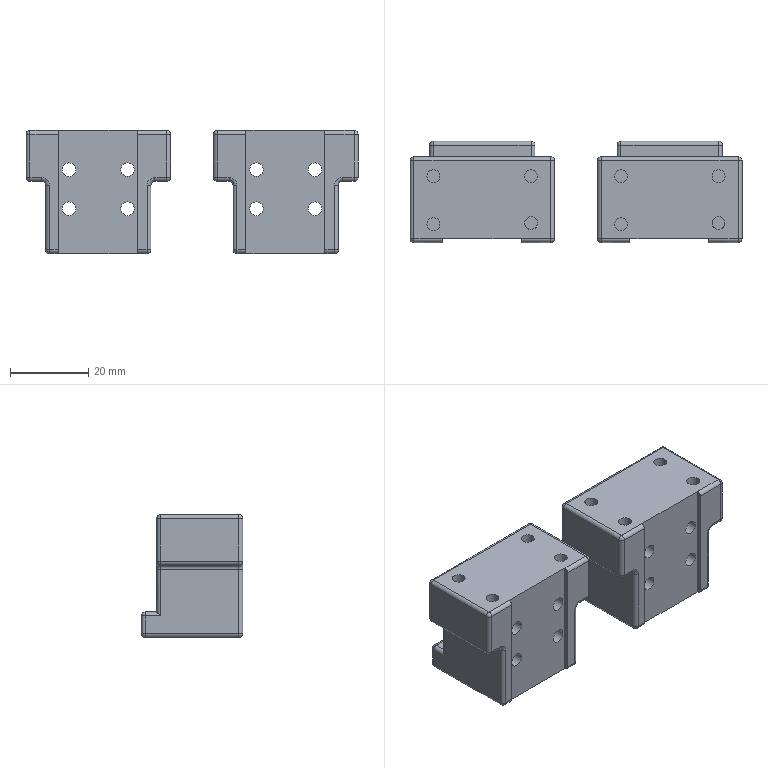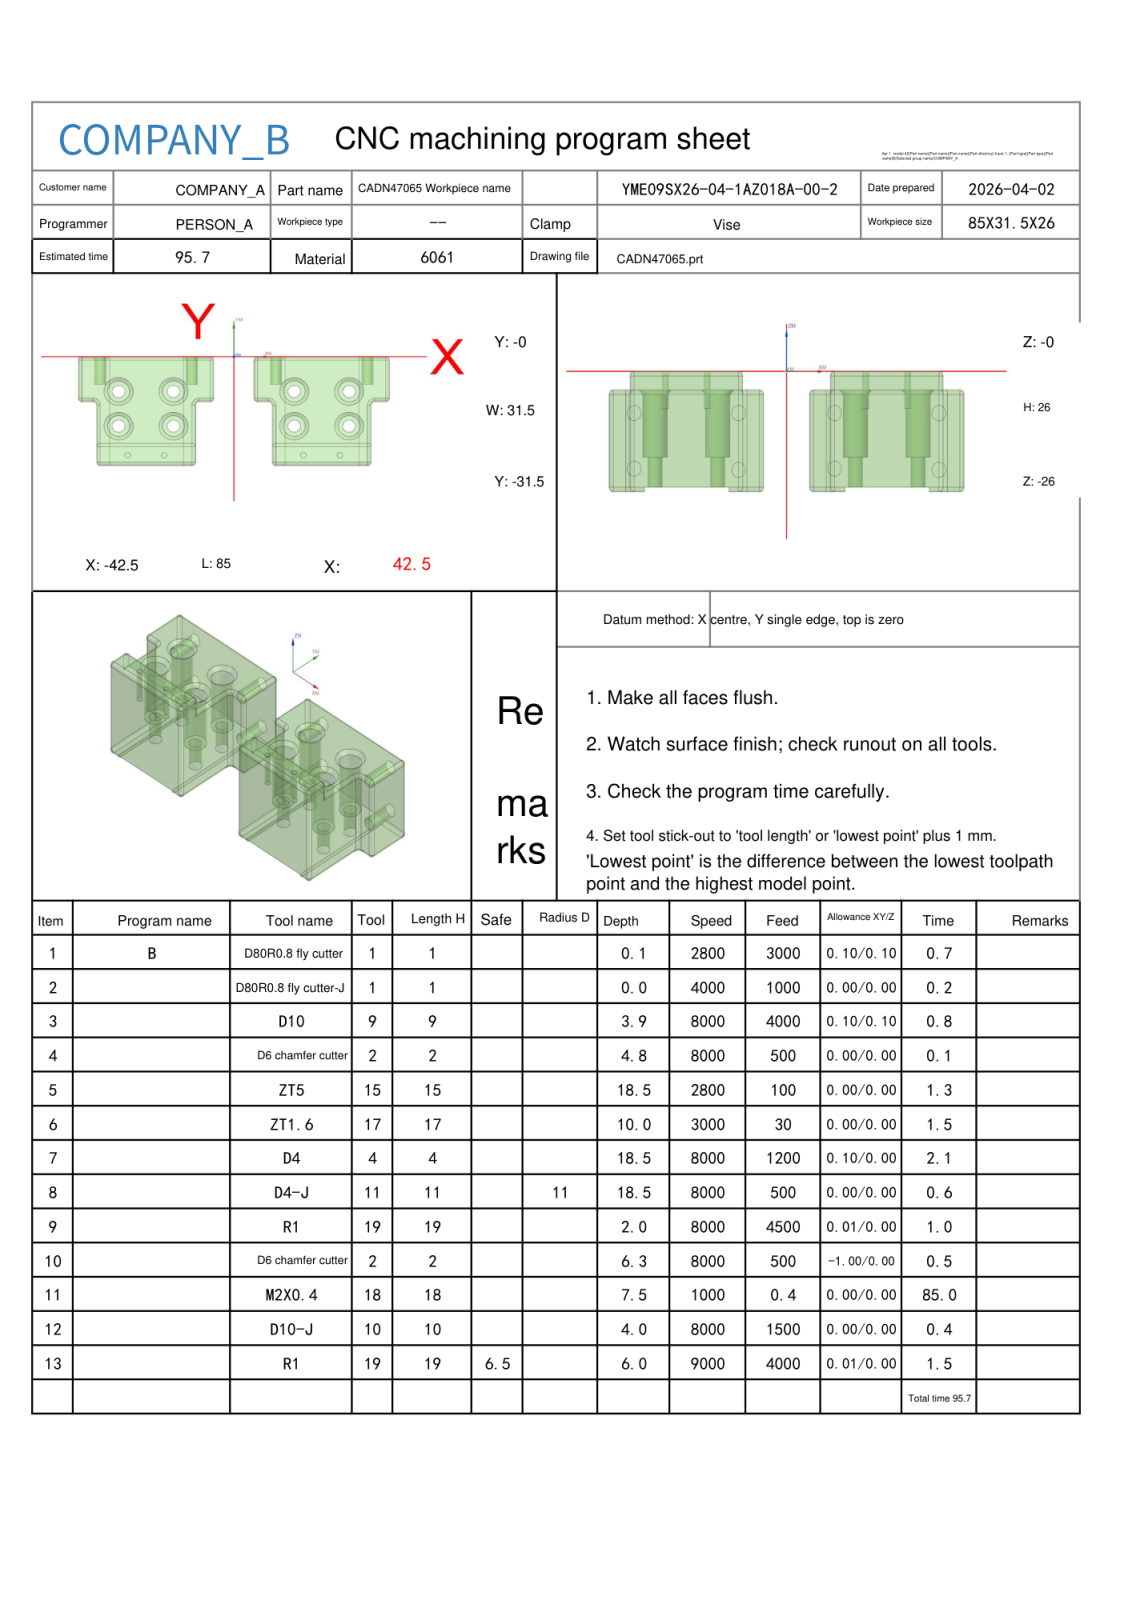NC program | NX | posted by the shop | part box 85 x 26 x 31.5 mm
Lines 1234 to 2575 of 12542:
N9 T19 M06
(R1  D=2. R=1. H=19 ce=0.01 di=0.00)
G00 G90 G54 X12.775 Y-25.799 M03 S8000
G43 H19 Z20.
M08
Z1.5
G01 X36.499 Z.257 F4500.
X36.539 Z.255
X36.614 Y-25.841 Z.25
X36.656 Y-25.916 Z.246
Y-25.955 Z.244
Y-30.5 Z.005
Y-30.54 Z.003
X36.613 Y-30.614 Z-.001
X36.538 Y-30.656 Z-.006
X36.498 Z-.008
X11.502
X11.5
G02 X11.344 Y-30.5 I0.0 J.156
G01 Y-25.955
G02 X11.5 Y-25.799 I.156 J0.0
G01 X36.499
G02 X36.656 Y-25.955 I0.0 J-.156
G01 Y-30.5
G02 X36.5 Y-30.656 I-.156 J0.0
G01 X36.498
X36.377 Y-30.686
X36.257
X36.137 Y-30.687
X36.017
X35.776 Y-30.688
X35.537
X35.056 Y-30.689
X34.575
X33.614 Y-30.692
X32.652 Y-30.694 Z-.009
X31.691 Y-30.696
X30.73 Y-30.698
X29.768 Y-30.7
X28.807 Y-30.702
X27.846 Y-30.704 Z-.01
X26.884 Y-30.707
X25.923 Y-30.708
X24.961 Y-30.711
X24. Y-30.712
X23.039 Y-30.714 Z-.011
X22.077 Y-30.716
X21.116 Y-30.718
X20.154 Y-30.72
X19.193 Y-30.721
X18.232 Y-30.724 Z-.012
X17.27 Y-30.725
X16.309 Y-30.727
X15.348 Y-30.728
X14.386 Y-30.731
X13.425 Y-30.732
X12.463 Y-30.734 Z-.013
X11.502 Y-30.735
X11.479
X11.456 Y-30.731
X11.434 Y-30.727
X11.412 Y-30.718
X11.391 Y-30.709
X11.371 Y-30.697
X11.351 Y-30.684
X11.335 Y-30.667
X11.318 Y-30.651
X11.305 Y-30.632
X11.292 Y-30.612
X11.283 Y-30.591
X11.274 Y-30.569
X11.269 Y-30.546
X11.264 Y-30.523
X11.263 Y-30.5
X11.265 Y-30.456
X11.267 Y-30.412
X11.264 Y-29.699
Y-28.985
X11.262 Y-28.228
Y-27.47 Z-.014
X11.26 Y-26.757
X11.259 Y-26.043
X11.258 Y-26.005
X11.259 Y-25.966
X11.255 Y-25.947
X11.258 Y-25.928
X11.263 Y-25.894
X11.275 Y-25.862
X11.284 Y-25.84
X11.297 Y-25.82
X11.311 Y-25.8
X11.328 Y-25.783
X11.345 Y-25.766
X11.365 Y-25.752
X11.385 Y-25.739
X11.407 Y-25.73
X11.429 Y-25.721
X11.453 Y-25.716
X11.476 Y-25.711
X11.5
X12.462 Y-25.709
X13.423 Y-25.708
X14.385 Y-25.706
X15.346 Y-25.704 Z-.015
X16.308 Y-25.703
X17.269 Y-25.701
X18.231 Y-25.699
X19.192 Y-25.697
X20.154 Y-25.696 Z-.016
X21.115 Y-25.694
X22.077 Y-25.693
X23.038 Y-25.691
X24. Y-25.69
X24.961 Y-25.689 Z-.017
X25.923 Y-25.687
X26.884 Y-25.686
X27.846 Y-25.684
X28.807 Y-25.691
X36.5 Z-.019
X36.525 Y-25.692
X36.551 Y-25.696
X36.576 Y-25.702
X36.601 Y-25.711
X36.624 Y-25.722
X36.647 Y-25.735
X36.668 Y-25.75
X36.687 Y-25.768
X36.704 Y-25.787
X36.72 Y-25.808
X36.733 Y-25.83
X36.744 Y-25.854
X36.753 Y-25.878
X36.76 Y-25.904
X36.763 Y-25.929
X36.765 Y-25.955
X36.761 Y-25.974
X36.749 Y-26.043
Y-30.412 Z-.02
X36.758 Y-30.488
X36.763 Y-30.529
X36.756 Y-30.566
X36.744 Y-30.602
X36.733 Y-30.626
X36.719 Y-30.648
X36.704 Y-30.669
X36.686 Y-30.688
X36.666 Y-30.706
X36.645 Y-30.721
X36.623 Y-30.735
X36.599 Y-30.745
X36.574 Y-30.754
X36.549 Y-30.76
X36.524 Y-30.764
X36.498 Y-30.765
X36.377 Y-30.792
X36.257
X36.137
X36.017
X35.777 Y-30.793
X35.537
X35.056 Y-30.794
X34.575 Y-30.796 Z-.021
X33.614 Y-30.797
X32.652 Y-30.799
X31.691 Y-30.801
X30.73 Y-30.803 Z-.022
X29.768 Y-30.804
X28.807 Y-30.807
X27.846 Y-30.808
X26.884 Y-30.81 Z-.023
X25.923 Y-30.812
X24.961 Y-30.814
X24. Y-30.815
X23.039 Y-30.817 Z-.024
X22.077 Y-30.819
X21.116 Y-30.821
X20.154 Y-30.822 Z-.025
X19.193 Y-30.824
X18.232 Y-30.826
X17.27 Y-30.827
X16.309 Y-30.829 Z-.026
X15.348 Y-30.831
X14.386 Y-30.832
X13.425 Y-30.834
X12.463 Y-30.835 Z-.027
X11.502 Y-30.837
X11.449 Y-30.833
X11.398 Y-30.821
X11.348 Y-30.802
X11.303 Y-30.774
X11.262 Y-30.74
X11.227 Y-30.699
X11.199 Y-30.654
X11.179 Y-30.605
X11.166 Y-30.553
X11.162 Y-30.5
X11.168 Y-30.456
Y-30.412
X11.166 Y-29.684
X11.165 Y-28.956 Z-.028
X11.164 Y-28.228
X11.162 Y-27.5
X11.161 Y-26.769
X11.159 Y-26.038
Y-25.988
X11.155 Y-25.939
X11.157 Y-25.917
X11.161 Y-25.886
X11.169 Y-25.855
X11.179 Y-25.825
X11.193 Y-25.797
X11.208 Y-25.769
X11.227 Y-25.743
X11.247 Y-25.719
X11.269 Y-25.697
X11.294 Y-25.677
X11.32 Y-25.66
X11.348 Y-25.644
X11.377 Y-25.632 Z-.029
X11.407 Y-25.622
X11.437 Y-25.615
X11.469 Y-25.61
X11.5 Y-25.609
X12.462 Y-25.608
X13.423 Y-25.606
X14.385 Y-25.605
X15.346 Y-25.603 Z-.03
X16.308 Y-25.602
X17.269 Y-25.599
X18.231 Y-25.598
X19.192 Y-25.596 Z-.031
X20.154 Y-25.595
X21.115 Y-25.593
X22.077 Y-25.592
X23.038 Y-25.591 Z-.032
X24. Y-25.589
X24.961 Y-25.588
X25.923 Y-25.586 Z-.033
X26.884 Y-25.585
X27.846 Y-25.583
X28.807 Y-25.582
X29.769 Y-25.58 Z-.034
X30.73 Y-25.579
X31.692 Y-25.577
X32.653 Y-25.576
X33.615 Y-25.574 Z-.035
X34.576 Y-25.573
X35.538 Y-25.572
X36.5 Y-25.57 Z-.036
X36.56 Y-25.575
X36.619 Y-25.589
X36.674 Y-25.612
X36.726 Y-25.643
X36.772 Y-25.682
X36.812 Y-25.728
X36.844 Y-25.78
X36.867 Y-25.836
X36.881 Y-25.895
X36.886 Y-25.955
X36.885 Y-25.972
X36.886 Y-26.008
X36.885 Y-26.044
X36.886 Y-26.772
X36.888 Y-27.5
Y-28.228
X36.881 Y-28.956 Z-.037
Y-30.412
X36.884 Y-30.437
X36.892 Y-30.461
Y-30.486
Y-30.51
X36.891 Y-30.527
X36.89 Y-30.543
X36.885 Y-30.579
X36.876 Y-30.614
X36.864 Y-30.648
X36.849 Y-30.681
X36.831 Y-30.712
X36.81 Y-30.741
X36.787 Y-30.769
X36.761 Y-30.794
X36.733 Y-30.817
X36.703 Y-30.837
X36.671 Y-30.854
X36.638 Y-30.868
X36.604 Y-30.879
X36.569 Y-30.887
X36.534 Y-30.892
X36.498 Y-30.894
X35.537 Y-30.895
X34.575 Y-30.897 Z-.038
X33.614 Y-30.898
X32.652 Y-30.9
X31.691 Y-30.902 Z-.039
X30.73 Y-30.903
X29.768 Y-30.905 Z-.04
X28.807 Y-30.907
X27.845 Y-30.908
X26.884 Y-30.91 Z-.041
X25.923 Y-30.912
X24.961 Y-30.913
X24. Y-30.915 Z-.042
X23.039 Y-30.916
X22.077 Y-30.918
X21.116 Y-30.92 Z-.043
X20.154 Y-30.922
X19.193 Y-30.923
X18.232 Y-30.925 Z-.044
X17.27 Y-30.926
X16.309 Y-30.928
X15.348 Y-30.93 Z-.045
X14.386 Y-30.931
X13.425 Y-30.933
X12.463 Y-30.935 Z-.046
X11.502 Y-30.936
X11.468 Y-30.935
X11.434 Y-30.931
X11.4 Y-30.925
X11.367 Y-30.915
X11.334 Y-30.904
X11.303 Y-30.89
X11.273 Y-30.873
X11.245 Y-30.854
X11.217 Y-30.833
X11.192 Y-30.81
X11.168 Y-30.785
X11.147 Y-30.757
X11.128 Y-30.729
X11.111 Y-30.699
X11.096 Y-30.668
X11.085 Y-30.635
X11.075 Y-30.602
X11.068 Y-30.569
X11.064 Y-30.534
X11.063 Y-30.5
X11.064 Y-30.456
Y-30.412
X11.063 Y-29.684 Z-.047
X11.062 Y-28.956
X11.061 Y-28.228
X11.06 Y-27.5
X11.059 Y-26.771 Z-.048
X11.058 Y-26.043
X11.057 Y-25.993
X11.055 Y-25.944
X11.058 Y-25.909
X11.062 Y-25.875
X11.07 Y-25.842
X11.08 Y-25.809
X11.092 Y-25.777
X11.107 Y-25.746
X11.125 Y-25.716
X11.144 Y-25.688
X11.166 Y-25.661
X11.189 Y-25.636
X11.215 Y-25.613
X11.242 Y-25.592
X11.271 Y-25.573
X11.301 Y-25.557
X11.332 Y-25.542
X11.365 Y-25.531
X11.398 Y-25.521
X11.432 Y-25.515
X11.466 Y-25.511
X11.5 Y-25.509
X12.462 Y-25.508
X13.423 Y-25.507 Z-.049
X14.385 Y-25.505
X15.346 Y-25.504
X16.308 Y-25.502 Z-.05
X17.269 Y-25.501
X18.231 Y-25.499
X19.192 Y-25.498 Z-.051
X20.154 Y-25.496
X21.115 Y-25.495 Z-.052
X22.077 Y-25.493
X23.038 Y-25.492
X24. Y-25.49 Z-.053
X24.961 Y-25.489
X25.923 Y-25.488
X26.884 Y-25.486 Z-.054
X27.846 Y-25.485
X28.807 Y-25.483
X29.769 Y-25.482 Z-.055
X30.73 Y-25.48
X31.692 Y-25.479
X32.653 Y-25.478 Z-.056
X33.615 Y-25.476
X34.576 Y-25.475
X35.538 Y-25.473 Z-.057
X36.5 Y-25.472
X36.537 Y-25.473
X36.575 Y-25.477
X36.613 Y-25.485
X36.649 Y-25.495
X36.685 Y-25.508
X36.719 Y-25.524
X36.753 Y-25.542
X36.784 Y-25.563
X36.814 Y-25.587
X36.842 Y-25.613
X36.868 Y-25.64
X36.892 Y-25.67
X36.913 Y-25.702
X36.932 Y-25.735
X36.948 Y-25.77
X36.961 Y-25.805
X36.971 Y-25.842
X36.979 Y-25.879
X36.983 Y-25.917
X36.985 Y-25.955
X36.98 Y-25.999
Y-26.043
X36.982 Y-26.771 Z-.058
X36.983 Y-27.5
X36.984 Y-28.228
X36.985 Y-28.956
X36.986 Y-29.684 Z-.059
X36.987 Y-30.412
Y-30.462
X36.991 Y-30.513
X36.989 Y-30.551
X36.984 Y-30.589
X36.975 Y-30.626
X36.964 Y-30.662
X36.95 Y-30.698
X36.934 Y-30.732
X36.914 Y-30.765
X36.893 Y-30.796
X36.869 Y-30.826
X36.842 Y-30.853
X36.814 Y-30.879
X36.784 Y-30.902
X36.752 Y-30.923
X36.718 Y-30.941
X36.684 Y-30.957
X36.648 Y-30.97
X36.611 Y-30.98
X36.574 Y-30.987
X36.536 Y-30.991
X36.498 Y-30.993
X35.537 Y-30.994 Z-.06
X34.575 Y-30.996
X33.614 Y-30.997
X32.652 Y-30.999 Z-.061
X31.691 Y-31.001
X30.73 Y-31.002 Z-.062
X29.768 Y-31.004
X28.807 Y-31.005
X27.845 Y-31.007 Z-.063
X26.884 Y-31.008
X25.923 Y-31.011 Z-.064
X24.961 Y-31.012
X24. Y-31.014 Z-.065
X23.039 Y-31.015
X22.077 Y-31.017
X21.116 Y-31.018 Z-.066
X20.154 Y-31.02
X19.193 Y-31.021 Z-.067
X18.232 Y-31.023
X17.27 Y-31.024
X16.309 Y-31.026 Z-.068
X15.348 Y-31.027
X14.386 Y-31.029 Z-.069
X13.425 Y-31.031
X12.463 Y-31.032
X11.502 Y-31.034 Z-.07
X11.467 Y-31.033
X11.432 Y-31.03
X11.398 Y-31.024
X11.364 Y-31.016
X11.33 Y-31.006
X11.297 Y-30.994
X11.265 Y-30.98
X11.234 Y-30.963
X11.204 Y-30.945
X11.176 Y-30.925
X11.148 Y-30.903
X11.123 Y-30.879
X11.099 Y-30.853
X11.076 Y-30.826
X11.056 Y-30.798
X11.037 Y-30.768
X11.021 Y-30.737
X11.006 Y-30.705
X10.993 Y-30.672
X10.983 Y-30.639
X10.975 Y-30.605
X10.97 Y-30.57
X10.966 Y-30.535
X10.965 Y-30.5
X10.967 Y-29.743 Z-.071
X10.965 Y-28.985
X10.964 Y-28.228
X10.963 Y-27.47 Z-.072
X10.962 Y-26.713
X10.958 Y-25.955
X10.959 Y-25.92
X10.962 Y-25.884
X10.968 Y-25.849
X10.976 Y-25.815
X10.986 Y-25.781
X10.999 Y-25.747
X11.013 Y-25.715
X11.03 Y-25.684
X11.049 Y-25.654
X11.069 Y-25.625
X11.092 Y-25.597
X11.116 Y-25.571
X11.142 Y-25.547
X11.169 Y-25.524
X11.198 Y-25.503
X11.229 Y-25.485
X11.26 Y-25.468
X11.292 Y-25.453
X11.326 Y-25.441
X11.36 Y-25.43 Z-.073
X11.394 Y-25.422
X11.429 Y-25.416
X11.465 Y-25.413
X11.5 Y-25.412
X12.462 Y-25.411
X13.423 Y-25.409
X14.385 Y-25.408 Z-.074
X15.346 Y-25.406
X16.308 Y-25.405 Z-.075
X17.269 Y-25.403
X18.231 Y-25.402
X19.192 Y-25.4 Z-.076
X20.154 Y-25.399
X21.115 Y-25.397 Z-.077
X22.077 Y-25.396
X23.038 Y-25.394 Z-.078
X24. Y-25.393
X24.961 Y-25.391
X25.923 Y-25.39 Z-.079
X26.884 Y-25.389
X27.846 Y-25.387 Z-.08
X28.807 Y-25.386
X29.769 Y-25.384
X30.73 Y-25.383 Z-.081
X31.692 Y-25.381
X32.653 Y-25.38 Z-.082
X33.615 Y-25.378
X34.576 Y-25.377 Z-.083
X35.538 Y-25.375
X36.5 Y-25.374
X36.538 Y-25.375
X36.575 Y-25.379
X36.613 Y-25.385
X36.65 Y-25.394
X36.687 Y-25.404
X36.722 Y-25.418
X36.757 Y-25.433
X36.79 Y-25.452
X36.823 Y-25.471
X36.854 Y-25.494 Z-.084
X36.883 Y-25.518
X36.911 Y-25.544
X36.937 Y-25.571
X36.961 Y-25.601
X36.984 Y-25.632
X37.004 Y-25.664
X37.022 Y-25.698
X37.038 Y-25.732
X37.051 Y-25.768
X37.062 Y-25.805
X37.071 Y-25.842
X37.077 Y-25.879
X37.081 Y-25.917
X37.083 Y-25.955
X37.084 Y-26.713
Y-27.47
X37.086 Y-28.228 Z-.085
X37.087 Y-28.985
X37.088 Y-29.743
X37.089 Y-30.5 Z-.086
X37.088 Y-30.539
X37.084 Y-30.577
X37.078 Y-30.615
X37.069 Y-30.653
X37.058 Y-30.69
X37.044 Y-30.726
X37.028 Y-30.761
X37.01 Y-30.795
X36.99 Y-30.828
X36.967 Y-30.86
X36.943 Y-30.89
X36.916 Y-30.918
X36.888 Y-30.944
X36.858 Y-30.969
X36.826 Y-30.991
X36.794 Y-31.012
X36.759 Y-31.03
X36.724 Y-31.046
X36.688 Y-31.059
X36.651 Y-31.071
X36.613 Y-31.079
X36.575 Y-31.086
X36.537 Y-31.089
X36.498 Y-31.09
X35.537 Y-31.092 Z-.087
X34.575 Y-31.094
X33.614 Y-31.095 Z-.088
X32.652 Y-31.097
X31.691 Y-31.098 Z-.089
X30.73 Y-31.1
X29.768 Y-31.101
X28.807 Y-31.103 Z-.09
X27.845 Y-31.104
X26.884 Y-31.106 Z-.091
X25.923 Y-31.107
X24.961 Y-31.109 Z-.092
X24. Y-31.11
X23.039 Y-31.112 Z-.093
X22.077 Y-31.113
X21.116 Y-31.115 Z-.094
X20.154 Y-31.116
X19.193 Y-31.118 Z-.095
X18.232 Y-31.119
X17.27 Y-31.121 Z-.096
X16.309 Y-31.122
X15.348 Y-31.124 Z-.097
X14.386 Y-31.125
X13.425 Y-31.127 Z-.098
X12.463 Y-31.128
X11.502 Y-31.13 Z-.099
X11.431 Y-31.127
X11.362 Y-31.115
X11.293 Y-31.096
X11.228 Y-31.069
X11.166 Y-31.035
X11.108 Y-30.994
X11.055 Y-30.947
X11.007 Y-30.894
X10.966 Y-30.836
X10.932 Y-30.774
X10.904 Y-30.709
X10.884 Y-30.641
X10.872 Y-30.57
X10.868 Y-30.498
X10.869 Y-30.455
X10.87 Y-30.412
X10.868 Y-29.699 Z-.1
Y-28.985
X10.867 Y-28.228
X10.865 Y-27.47 Z-.101
X10.864 Y-26.757
X10.863 Y-26.043
Y-26.
X10.861 Y-25.957
X10.862 Y-25.929
X10.867 Y-25.87
X10.877 Y-25.813 Z-.102
X10.897 Y-25.744
X10.924 Y-25.678
X10.959 Y-25.615
X11. Y-25.556
X11.048 Y-25.503
X11.101 Y-25.455
X11.16 Y-25.414
X11.223 Y-25.379
X11.289 Y-25.351
X11.358 Y-25.331
X11.428 Y-25.319
X11.5 Y-25.315
X12.462 Y-25.314
X13.423 Y-25.312 Z-.103
X14.385 Y-25.311
X15.346 Y-25.309 Z-.104
X16.308 Y-25.308
X17.269 Y-25.307 Z-.105
X18.231 Y-25.305
X19.192 Y-25.304 Z-.106
X20.154 Y-25.302
X21.115 Y-25.301 Z-.107
X22.077 Y-25.299
X23.038 Y-25.298 Z-.108
X24. Y-25.296
X24.961 Y-25.295 Z-.109
X25.923 Y-25.294
X26.884 Y-25.293 Z-.11
X27.846 Y-25.291
X28.807 Y-25.29 Z-.111
X29.769 Y-25.288
X30.73 Y-25.287 Z-.112
X31.692 Y-25.285
X32.653 Y-25.284 Z-.113
X33.615 Y-25.282
X34.577 Y-25.281 Z-.114
X35.538 Y-25.28
X36.5 Y-25.279 Z-.115
X36.575 Y-25.283
X36.65 Y-25.295
X36.723 Y-25.316
X36.793 Y-25.345
X36.86 Y-25.382
X36.922 Y-25.425
X36.979 Y-25.476
X37.03 Y-25.533
X37.074 Y-25.595
X37.111 Y-25.661
X37.14 Y-25.731
X37.161 Y-25.804
X37.174 Y-25.879
X37.178 Y-25.955
X37.175 Y-25.999
Y-26.043
X37.176 Y-26.757
X37.177 Y-27.47 Z-.116
X37.178 Y-28.228
X37.179 Y-28.985 Z-.117
X37.18 Y-29.699
X37.181 Y-30.412
Y-30.454
X37.185 Y-30.497
X37.184 Y-30.513
Y-30.529
X37.179 Y-30.591
X37.168 Y-30.653
X37.147 Y-30.727
X37.117 Y-30.798
X37.08 Y-30.865 Z-.118
X37.035 Y-30.928
X36.984 Y-30.986
X36.927 Y-31.037
X36.864 Y-31.081
X36.796 Y-31.119
X36.725 Y-31.148
X36.651 Y-31.169
X36.575 Y-31.182
X36.498 Y-31.186
X35.537 Y-31.188
X34.575 Y-31.189 Z-.119
X33.614 Y-31.191 Z-.12
X32.652 Y-31.192
X31.691 Y-31.194 Z-.121
X30.73 Y-31.195
X29.768 Y-31.197 Z-.122
X28.807 Y-31.198
X27.845 Y-31.2 Z-.123
X26.884 Y-31.201
X25.923 Y-31.203 Z-.124
X24.961 Y-31.204
X24. Y-31.206 Z-.125
X23.039 Y-31.207 Z-.126
X22.077 Y-31.209
X21.116 Y-31.21 Z-.127
X20.154 Y-31.212
X19.193 Y-31.213 Z-.128
X18.232 Y-31.215
X17.27 Y-31.216 Z-.129
X16.309 Y-31.218
X15.348 Y-31.219 Z-.13
X14.386 Y-31.22 Z-.131
X13.425 Y-31.222
X12.463 Y-31.223 Z-.132
X11.502 Y-31.225
X11.421 Y-31.221
X11.34 Y-31.207
X11.262 Y-31.185
X11.187 Y-31.154
X11.115 Y-31.115
X11.049 Y-31.068
X10.988 Y-31.014
X10.933 Y-30.953 Z-.133
X10.886 Y-30.887
X10.846 Y-30.815
X10.815 Y-30.74
X10.792 Y-30.662
X10.778 Y-30.581
X10.774 Y-30.5
X10.775 Y-30.456
Y-30.412
X10.774 Y-29.684
X10.773 Y-28.956 Z-.134
X10.772 Y-28.228
X10.771 Y-27.5 Z-.135
X10.769 Y-26.771
X10.768 Y-26.043
Y-25.998
X10.767 Y-25.954
Y-25.925
X10.775 Y-25.845
X10.791 Y-25.766 Z-.136
X10.816 Y-25.69
X10.849 Y-25.617
X10.889 Y-25.548
X10.937 Y-25.484
X10.992 Y-25.426
X11.052 Y-25.373
X11.118 Y-25.328
X11.189 Y-25.29
X11.263 Y-25.26
X11.34 Y-25.238
X11.42 Y-25.225
X11.5 Y-25.22
X12.461 Y-25.219 Z-.137
X13.423 Y-25.218
X14.384 Y-25.216 Z-.138
X15.346 Y-25.215
X16.307 Y-25.213 Z-.139
X17.269 Y-25.212
X18.23 Y-25.211 Z-.14
X19.192 Y-25.209
X20.153 Y-25.208 Z-.141
X21.115 Y-25.207 Z-.142
X22.077 Y-25.205
X23.038 Y-25.204 Z-.143
X24. Y-25.202
X24.961 Y-25.201 Z-.144
X25.923 Y-25.199
X26.884 Y-25.198 Z-.145
X27.846 Y-25.197
X28.807 Y-25.196 Z-.146
X29.769 Y-25.194
X30.73 Y-25.193 Z-.147
X31.692 Y-25.191 Z-.148
X32.653 Y-25.19
X33.615 Y-25.189 Z-.149
X34.576 Y-25.188
X35.538 Y-25.186 Z-.15
X36.5 Y-25.185
X36.586 Y-25.189
X36.671 Y-25.204
X36.754 Y-25.227
X36.834 Y-25.261 Z-.151
X36.91 Y-25.302
X36.981 Y-25.352
X37.045 Y-25.41
X37.103 Y-25.474
X37.153 Y-25.545
X37.195 Y-25.62
X37.229 Y-25.7
X37.253 Y-25.783
X37.267 Y-25.869
X37.272 Y-25.955
Y-25.999
Y-26.043
X37.274 Y-26.771
Y-27.5 Z-.152
X37.276 Y-28.228
Y-28.956 Z-.153
X37.278 Y-29.684
X37.279 Y-30.412 Z-.154
Y-30.456
Y-30.5
X37.278 Y-30.516
Y-30.533
X37.27 Y-30.617
X37.253 Y-30.701
X37.226 Y-30.782
X37.191 Y-30.86
X37.148 Y-30.933
X37.097 Y-31.001
X37.039 Y-31.063
X36.974 Y-31.119
X36.904 Y-31.167
X36.828 Y-31.207
X36.749 Y-31.239
X36.667 Y-31.262
X36.583 Y-31.276
X36.498 Y-31.28
X35.537 Y-31.282 Z-.155
X34.575 Y-31.283 Z-.156
X33.614 Y-31.285
X32.652 Y-31.286 Z-.157
X31.691 Y-31.288
X30.73 Y-31.289 Z-.158
X29.768 Y-31.29 Z-.159
X28.807 Y-31.292
X27.845 Y-31.293 Z-.16
X26.884 Y-31.295
X25.923 Y-31.296 Z-.161
X24.961 Y-31.297 Z-.162
X24. Y-31.299
X23.039 Y-31.3 Z-.163
X22.077 Y-31.302 Z-.164
X21.116 Y-31.303
X20.154 Y-31.305 Z-.165
X19.193 Y-31.306
X18.232 Y-31.308 Z-.166
X17.27 Y-31.309 Z-.167
X16.309 Y-31.31
X15.347 Y-31.312 Z-.168
X14.386 Y-31.313
X13.425 Y-31.314 Z-.169
X12.463 Y-31.316 Z-.17
X11.502 Y-31.317
X11.456 Y-31.316
X11.41 Y-31.312
X11.365 Y-31.306
X11.32 Y-31.297
X11.275 Y-31.286
X11.231 Y-31.272
X11.188 Y-31.256
X11.147 Y-31.237
X11.106 Y-31.217 Z-.171
X11.066 Y-31.193
X11.028 Y-31.168
X10.991 Y-31.14
X10.956 Y-31.111
X10.922 Y-31.079
X10.89 Y-31.046
X10.861 Y-31.011
X10.833 Y-30.974
X10.807 Y-30.936
X10.784 Y-30.897
X10.763 Y-30.856
X10.744 Y-30.814
X10.727 Y-30.771
X10.713 Y-30.727
X10.702 Y-30.682
X10.693 Y-30.637
X10.686 Y-30.592
X10.682 Y-30.546
X10.681 Y-30.5
Y-29.743 Z-.172
X10.68 Y-28.985
X10.679 Y-28.228 Z-.173
X10.678 Y-27.47
X10.677 Y-26.713
X10.674 Y-25.955 Z-.174
X10.675 Y-25.909
X10.679 Y-25.863
X10.686 Y-25.817
X10.695 Y-25.771
X10.706 Y-25.727
X10.72 Y-25.682
X10.737 Y-25.639
X10.756 Y-25.597
X10.777 Y-25.555
X10.8 Y-25.515
X10.826 Y-25.477
X10.854 Y-25.44
X10.884 Y-25.404
X10.916 Y-25.371
X10.949 Y-25.339
X10.985 Y-25.309
X11.022 Y-25.281
X11.06 Y-25.255
X11.1 Y-25.231 Z-.175
X11.141 Y-25.21
X11.184 Y-25.191
X11.227 Y-25.174
X11.271 Y-25.16
X11.316 Y-25.149
X11.362 Y-25.139
X11.408 Y-25.133
X11.454 Y-25.129
X11.5 Y-25.128
X12.462 Y-25.126
X13.423 Y-25.125 Z-.176
X14.385 Y-25.124 Z-.177
X15.346 Y-25.122
X16.308 Y-25.121 Z-.178
X17.269 Y-25.12
X18.231 Y-25.118 Z-.179
X19.192 Y-25.117 Z-.18
X20.154 Y-25.116
X21.115 Y-25.114 Z-.181
X22.077 Y-25.113 Z-.182
X23.038 Y-25.112
X24. Y-25.11 Z-.183
X24.961 Y-25.109
X25.923 Y-25.107 Z-.184
X26.884 Y-25.106 Z-.185
X27.846 Y-25.105
X28.807 Y-25.104 Z-.186
X29.769 Y-25.102
X30.73 Y-25.101 Z-.187
X31.692 Y-25.099 Z-.188
X32.653
X33.615 Y-25.097 Z-.189
X34.577 Y-25.096
X35.538 Y-25.094 Z-.19
X36.5 Y-25.093 Z-.191
X36.548 Y-25.094
X36.596 Y-25.098
X36.644 Y-25.105
X36.691 Y-25.114
X36.738 Y-25.126
X36.784 Y-25.141
X36.83 Y-25.158
X36.874 Y-25.178
X36.917 Y-25.2
X36.959 Y-25.225
X36.999 Y-25.251
X37.038 Y-25.281
X37.075 Y-25.312
X37.11 Y-25.345
X37.144 Y-25.38
X37.175 Y-25.417
X37.204 Y-25.456
X37.231 Y-25.496
X37.256 Y-25.537
X37.278 Y-25.581
X37.298 Y-25.625
X37.315 Y-25.67
X37.33 Y-25.716
X37.342 Y-25.763
X37.352 Y-25.811
X37.358 Y-25.859 Z-.192
X37.363 Y-25.907
X37.364 Y-25.955
X37.363 Y-26.713
X37.364 Y-27.47 Z-.193
X37.365 Y-28.228
X37.366 Y-28.985 Z-.194
X37.367 Y-29.743
X37.37 Y-30.5
X37.369 Y-30.549 Z-.195
X37.365 Y-30.598
X37.358 Y-30.646
X37.349 Y-30.694
X37.336 Y-30.741
X37.322 Y-30.788
X37.304 Y-30.834
X37.284 Y-30.878
X37.262 Y-30.922
X37.237 Y-30.964
X37.21 Y-31.005
X37.18 Y-31.044
X37.149 Y-31.081
X37.115 Y-31.117
X37.08 Y-31.15
X37.042 Y-31.182
X37.003 Y-31.211
X36.962 Y-31.239
X36.92 Y-31.263
X36.877 Y-31.286
X36.832 Y-31.306
X36.786 Y-31.323
X36.74 Y-31.338
X36.692 Y-31.35
X36.644 Y-31.36
X36.596 Y-31.367
X36.547 Y-31.371
X36.498 Y-31.372
X35.537 Y-31.373 Z-.196
X34.575 Y-31.375 Z-.197
X33.614 Y-31.376
X32.652 Y-31.378 Z-.198
X31.691 Y-31.379 Z-.199
X30.73 Y-31.38
X29.768 Y-31.382 Z-.2
X28.807 Y-31.383 Z-.201
X27.845 Y-31.385
X26.884 Y-31.386 Z-.202
X25.923 Y-31.387 Z-.203
X24.961 Y-31.388
X24. Y-31.39 Z-.204
X23.039 Y-31.391 Z-.205
X22.077 Y-31.393
X21.116 Y-31.394 Z-.206
X20.154 Y-31.396 Z-.207
X19.193 Y-31.397
X18.232 Y-31.398 Z-.208
X17.27 Y-31.399 Z-.209
X16.309 Y-31.401
X15.347 Y-31.402 Z-.21
X14.386 Y-31.404 Z-.211
X13.425 Y-31.405 Z-.212
X12.463 Y-31.406
X11.502 Y-31.408 Z-.213
X11.413 Y-31.404
X11.325 Y-31.391
X11.238 Y-31.369
X11.154 Y-31.34
X11.073 Y-31.302
X10.996 Y-31.256
X10.924 Y-31.203
X10.858 Y-31.143
X10.798 Y-31.077
X10.745 Y-31.006
X10.699 Y-30.929 Z-.214
X10.66 Y-30.848
X10.63 Y-30.764
X10.608 Y-30.678
X10.595 Y-30.589
X10.59 Y-30.5
X10.591 Y-30.456
Y-30.412
X10.59 Y-29.699
X10.589 Y-28.985 Z-.215
X10.588 Y-28.228
X10.587 Y-27.47 Z-.216
X10.586 Y-26.757
X10.585 Y-26.043 Z-.217
Y-26.
X10.584 Y-25.937
X10.589 Y-25.856
X10.601 Y-25.777
X10.623 Y-25.689
X10.653 Y-25.604
X10.692 Y-25.523
X10.738 Y-25.446
X10.791 Y-25.374
X10.852 Y-25.307 Z-.218
X10.918 Y-25.246
X10.991 Y-25.192
X11.068 Y-25.146
X11.149 Y-25.107
X11.234 Y-25.077
X11.321 Y-25.055
X11.41 Y-25.042
X11.5 Y-25.037
X12.462 Y-25.036 Z-.219
X13.423 Y-25.035
X14.385 Y-25.033 Z-.22
X15.346 Y-25.032 Z-.221
X16.308 Y-25.031
X17.269 Y-25.03 Z-.222
X18.231 Y-25.028 Z-.223
X19.192 Y-25.027
X20.154 Y-25.026 Z-.224
X21.115 Y-25.024 Z-.225
X22.077 Y-25.023
X23.038 Y-25.022 Z-.226
X24. Y-25.02 Z-.227
X24.961 Y-25.019
X25.923 Y-25.018 Z-.228
X26.884 Y-25.017 Z-.229
X27.846 Y-25.015 Z-.23
X28.807 Y-25.014
X29.769 Y-25.013 Z-.231
X30.73 Y-25.012 Z-.232
X31.692 Y-25.01
X32.654 Y-25.009 Z-.233
X33.615 Y-25.008 Z-.234
X34.577 Y-25.006
X35.538 Y-25.005 Z-.235
X36.5 Y-25.004 Z-.236
X36.593 Y-25.008
X36.685 Y-25.022
X36.776 Y-25.044
X36.864 Y-25.076
X36.949 Y-25.115
X37.029 Y-25.163
X37.104 Y-25.219
X37.173 Y-25.282
X37.236 Y-25.351
X37.292 Y-25.426
X37.34 Y-25.506
X37.38 Y-25.591
X37.412 Y-25.679
X37.435 Y-25.769
X37.449 Y-25.862 Z-.237
X37.454 Y-25.955
Y-25.999
X37.453 Y-26.043
X37.455 Y-26.757
Y-27.47 Z-.238
X37.457 Y-28.228
Y-28.985 Z-.239
X37.458 Y-29.699
X37.459 Y-30.412 Z-.24
Y-30.454
Y-30.52
X37.454 Y-30.604
X37.441 Y-30.687
X37.418 Y-30.779
X37.387 Y-30.868
X37.346 Y-30.953
X37.298 Y-31.034
X37.242 Y-31.11
X37.178 Y-31.18
X37.108 Y-31.243
X37.033 Y-31.3
X36.952 Y-31.348 Z-.241
X36.866 Y-31.388
X36.777 Y-31.42
X36.686 Y-31.443
X36.592 Y-31.457
X36.498 Y-31.462
X35.537 Y-31.463 Z-.242
X34.575 Y-31.464
X33.614 Y-31.466 Z-.243
X32.652 Y-31.467 Z-.244
X31.691 Y-31.468 Z-.245
X30.73 Y-31.469
X29.768 Y-31.471 Z-.246
X28.807 Y-31.472 Z-.247
X27.845 Y-31.474
X26.884 Y-31.475 Z-.248
X25.923 Y-31.476 Z-.249
X24.961 Y-31.477 Z-.25
X24. Y-31.479
X23.039 Y-31.48 Z-.251
X22.077 Y-31.482 Z-.252
X21.116 Z-.253
X20.154 Y-31.484
X19.193 Y-31.485 Z-.254
X18.232 Y-31.487 Z-.255
X17.27 Y-31.488
X16.309 Y-31.489 Z-.256
X15.347 Y-31.49 Z-.257
X14.386 Y-31.492 Z-.258
X13.425 Y-31.493
X12.463 Y-31.495 Z-.259
X11.502 Y-31.496 Z-.26
X11.453 Y-31.495
X11.404 Y-31.491
X11.356 Y-31.486
X11.307 Y-31.477
X11.26 Y-31.467
X11.212 Y-31.454
X11.166 Y-31.439
X11.12 Y-31.421
X11.075 Y-31.401
X11.032 Y-31.379
X10.989 Y-31.355
X10.947 Y-31.329
X10.907 Y-31.301
X10.869 Y-31.271
X10.831 Y-31.239
X10.796 Y-31.205
X10.762 Y-31.17 Z-.261
X10.73 Y-31.133
X10.7 Y-31.095
X10.671 Y-31.055
X10.645 Y-31.013
X10.621 Y-30.971
X10.599 Y-30.927
X10.579 Y-30.882
X10.561 Y-30.836
X10.546 Y-30.79
X10.532 Y-30.743
X10.522 Y-30.695
X10.513 Y-30.647
X10.507 Y-30.598
X10.503 Y-30.549
X10.502 Y-30.5
X10.503 Y-30.456
Y-30.412
X10.502 Y-29.684 Z-.262
X10.501 Y-28.956
X10.5 Y-28.228 Z-.263
Y-27.5
X10.499 Y-26.771 Z-.264
X10.498 Y-26.043
Y-25.998 Z-.265
X10.496 Y-25.935
X10.503 Y-25.838
X10.519 Y-25.742
X10.544 Y-25.648
X10.578 Y-25.557
X10.621 Y-25.469
X10.672 Y-25.386
X10.73 Y-25.309
X10.796 Y-25.237
X10.869 Y-25.173
X10.948 Y-25.115
X11.032 Y-25.066
X11.12 Y-25.024
X11.212 Y-24.992 Z-.266
X11.306 Y-24.968
X11.402 Y-24.954
X11.5 Y-24.949
X12.461 Y-24.948
X13.423 Y-24.947 Z-.267
X14.384 Y-24.945 Z-.268
X15.346 Y-24.944 Z-.269
X16.307 Y-24.943
X17.269 Y-24.942 Z-.27
X18.23 Y-24.94 Z-.271
X19.192 Y-24.939 Z-.272
X20.153 Y-24.938
X21.115 Y-24.937 Z-.273
X22.077 Y-24.935 Z-.274
X23.038 Y-24.934 Z-.275
X24. Y-24.933
X24.961 Y-24.932 Z-.276
X25.923 Y-24.93 Z-.277
X26.884 Y-24.929
X27.846 Y-24.928 Z-.278
X28.807 Y-24.927 Z-.279
X29.769 Y-24.925 Z-.28
X30.73 Y-24.924
X31.692 Y-24.923 Z-.281
X32.653 Y-24.922 Z-.282
X33.615 Y-24.92 Z-.283
X34.576 Y-24.919
X35.538 Y-24.918 Z-.284
X36.5 Y-24.917 Z-.285
X36.551 Y-24.918
X36.601 Y-24.922
X36.652 Y-24.928
X36.702 Y-24.937
X36.752 Y-24.947
X36.801 Y-24.961
X36.85 Y-24.977
X36.897 Y-24.995
X36.944 Y-25.016
X36.989 Y-25.039
X37.034 Y-25.064
X37.077 Y-25.091
X37.119 Y-25.12
X37.159 Y-25.152
X37.198 Y-25.185
X37.235 Y-25.22
X37.27 Y-25.257
X37.303 Y-25.296
X37.335 Y-25.336 Z-.286
X37.364 Y-25.378
X37.392 Y-25.421
X37.417 Y-25.465
X37.44 Y-25.511
X37.461 Y-25.557
X37.479 Y-25.605
X37.495 Y-25.653
X37.509 Y-25.702
X37.52 Y-25.752
X37.529 Y-25.803
X37.535 Y-25.853
X37.539 Y-25.904
X37.541 Y-25.955
X37.538 Y-25.999
X37.541 Y-28.228 Z-.288
X37.542 Y-28.956
X37.543 Y-29.684 Z-.289
X37.544 Y-30.412
Y-30.456
X37.546 Y-30.5
Y-30.521 Z-.29
X37.539 Y-30.623
X37.523 Y-30.723
X37.496 Y-30.821
X37.461 Y-30.916
X37.416 Y-31.007
X37.363 Y-31.093
X37.301 Y-31.174
X37.232 Y-31.249
X37.156 Y-31.316
X37.074 Y-31.376
X36.987 Y-31.428
X36.895 Y-31.471
X36.799 Y-31.505 Z-.291
X36.7 Y-31.529
X36.6 Y-31.544
X36.498 Y-31.548
X35.537 Y-31.55 Z-.292